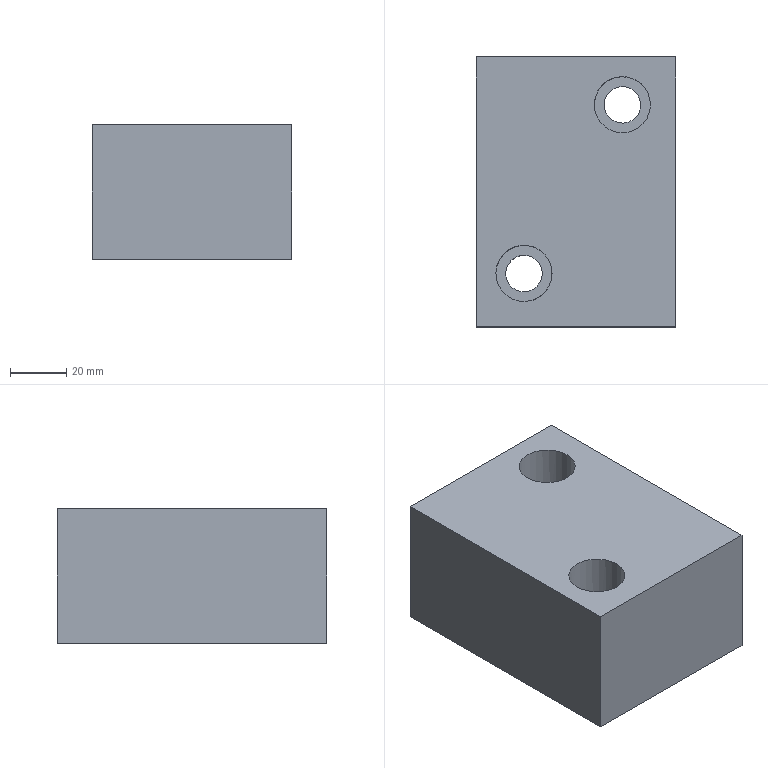Part | STEP file | gslz 2016.10.28-13_id770_x_t | 1 solid | 12 faces | box 71 x 96 x 48 mm | volume 304991 mm3 | plane 8 | cylinder 4 | commonest cylinder face diameters 13 x2 20 x2
STEP:
#1=CARTESIAN_POINT('',(0.,0.,0.));
#2=DIRECTION('',(0.,0.,1.));
#3=DIRECTION('',(1.,0.,0.));
#4=AXIS2_PLACEMENT_3D('',#1,#2,#3);
#5=CARTESIAN_POINT('',(-1464.591,-78.908,-48.));
#6=VERTEX_POINT('',#5);
#7=CARTESIAN_POINT('',(-1463.5,-72.5,-48.));
#8=DIRECTION('',(0.,0.,1.));
#9=DIRECTION('',(-0.1678,-0.9858,0.));
#10=AXIS2_PLACEMENT_3D('',#7,#8,#9);
#11=CIRCLE('',#10,6.5);
#12=CARTESIAN_POINT('',(-1613.5,-26.,-48.));
#13=DIRECTION('',(0.,0.,1.));
#14=DIRECTION('',(0.,1.,0.));
#15=AXIS2_PLACEMENT_3D('',#12,#13,#14);
#16=PLANE('',#15);
#17=CARTESIAN_POINT('',(-46.5,-150.));
#18=DIRECTION('',(-0.9858,0.1678));
#19=AXIS2_PLACEMENT_2D('',#17,#18);
#20=CIRCLE('',#19,6.5);
#21=(GEOMETRIC_REPRESENTATION_CONTEXT(2)PARAMETRIC_REPRESENTATION_CONTEXT()REPRESENTATION_CONTEXT('',''));
#22=DEFINITIONAL_REPRESENTATION('',(#20),#21);
#23=PCURVE('',#16,#22);
#24=CARTESIAN_POINT('',(-1463.5,-72.5,-8.541));
#25=DIRECTION('',(0.,0.,-1.));
#26=DIRECTION('',(-1.,0.,0.));
#27=AXIS2_PLACEMENT_3D('',#24,#25,#26);
#28=CYLINDRICAL_SURFACE('',#27,6.5);
#29=CARTESIAN_POINT('',(11.164,39.459));
#30=DIRECTION('',(-1.,0.));
#31=VECTOR('',#30,1.);
#32=LINE('',#29,#31);
#33=(GEOMETRIC_REPRESENTATION_CONTEXT(2)PARAMETRIC_REPRESENTATION_CONTEXT()REPRESENTATION_CONTEXT('',''));
#34=DEFINITIONAL_REPRESENTATION('',(#32),#33);
#35=PCURVE('',#28,#34);
#36=SURFACE_CURVE('',#11,(#23,#35),.PCURVE_S1.);
#37=EDGE_CURVE('',#6,#6,#36,.T.);
#38=ORIENTED_EDGE('',*,*,#37,.T.);
#39=EDGE_LOOP('',(#38));
#40=FACE_BOUND('',#39,.T.);
#41=CARTESIAN_POINT('',(-1429.591,-18.908,-48.));
#42=VERTEX_POINT('',#41);
#43=CARTESIAN_POINT('',(-1428.5,-12.5,-48.));
#44=DIRECTION('',(0.,0.,1.));
#45=DIRECTION('',(-0.1678,-0.9858,0.));
#46=AXIS2_PLACEMENT_3D('',#43,#44,#45);
#47=CIRCLE('',#46,6.5);
#48=CARTESIAN_POINT('',(13.5,-185.));
#49=DIRECTION('',(-0.9858,0.1678));
#50=AXIS2_PLACEMENT_2D('',#48,#49);
#51=CIRCLE('',#50,6.5);
#52=(GEOMETRIC_REPRESENTATION_CONTEXT(2)PARAMETRIC_REPRESENTATION_CONTEXT()REPRESENTATION_CONTEXT('',''));
#53=DEFINITIONAL_REPRESENTATION('',(#51),#52);
#54=PCURVE('',#16,#53);
#55=CARTESIAN_POINT('',(-1428.5,-12.5,-8.541));
#56=DIRECTION('',(0.,0.,-1.));
#57=DIRECTION('',(-1.,0.,0.));
#58=AXIS2_PLACEMENT_3D('',#55,#56,#57);
#59=CYLINDRICAL_SURFACE('',#58,6.5);
#60=CARTESIAN_POINT('',(11.164,39.459));
#61=DIRECTION('',(-1.,0.));
#62=VECTOR('',#61,1.);
#63=LINE('',#60,#62);
#64=(GEOMETRIC_REPRESENTATION_CONTEXT(2)PARAMETRIC_REPRESENTATION_CONTEXT()REPRESENTATION_CONTEXT('',''));
#65=DEFINITIONAL_REPRESENTATION('',(#63),#64);
#66=PCURVE('',#59,#65);
#67=SURFACE_CURVE('',#47,(#54,#66),.PCURVE_S1.);
#68=EDGE_CURVE('',#42,#42,#67,.T.);
#69=ORIENTED_EDGE('',*,*,#68,.T.);
#70=EDGE_LOOP('',(#69));
#71=FACE_BOUND('',#70,.T.);
#72=CARTESIAN_POINT('',(-1480.5,-91.5,-48.));
#73=VERTEX_POINT('',#72);
#74=CARTESIAN_POINT('',(-1409.5,-91.5,-48.));
#75=VERTEX_POINT('',#74);
#76=CARTESIAN_POINT('',(-1613.5,-91.5,-48.));
#77=DIRECTION('',(1.,0.,0.));
#78=VECTOR('',#77,1.);
#79=LINE('',#76,#78);
#80=CARTESIAN_POINT('',(-65.5,0.));
#81=DIRECTION('',(0.,-1.));
#82=VECTOR('',#81,1.);
#83=LINE('',#80,#82);
#84=(GEOMETRIC_REPRESENTATION_CONTEXT(2)PARAMETRIC_REPRESENTATION_CONTEXT()REPRESENTATION_CONTEXT('',''));
#85=DEFINITIONAL_REPRESENTATION('',(#83),#84);
#86=PCURVE('',#16,#85);
#87=CARTESIAN_POINT('',(-1608.5,-91.5,-43.));
#88=DIRECTION('',(0.,-1.,0.));
#89=DIRECTION('',(0.,0.,1.));
#90=AXIS2_PLACEMENT_3D('',#87,#88,#89);
#91=PLANE('',#90);
#92=CARTESIAN_POINT('',(-5.,5.));
#93=DIRECTION('',(0.,-1.));
#94=VECTOR('',#93,1.);
#95=LINE('',#92,#94);
#96=(GEOMETRIC_REPRESENTATION_CONTEXT(2)PARAMETRIC_REPRESENTATION_CONTEXT()REPRESENTATION_CONTEXT('',''));
#97=DEFINITIONAL_REPRESENTATION('',(#95),#96);
#98=PCURVE('',#91,#97);
#99=SURFACE_CURVE('',#79,(#86,#98),.PCURVE_S1.);
#100=EDGE_CURVE('',#73,#75,#99,.T.);
#101=ORIENTED_EDGE('',*,*,#100,.F.);
#102=CARTESIAN_POINT('',(-1480.5,4.5,-48.));
#103=VERTEX_POINT('',#102);
#104=CARTESIAN_POINT('',(-1480.5,-43.5,-48.));
#105=DIRECTION('',(0.,-1.,0.));
#106=VECTOR('',#105,1.);
#107=LINE('',#104,#106);
#108=CARTESIAN_POINT('',(-17.5,-133.));
#109=DIRECTION('',(-1.,0.));
#110=VECTOR('',#109,1.);
#111=LINE('',#108,#110);
#112=(GEOMETRIC_REPRESENTATION_CONTEXT(2)PARAMETRIC_REPRESENTATION_CONTEXT()REPRESENTATION_CONTEXT('',''));
#113=DEFINITIONAL_REPRESENTATION('',(#111),#112);
#114=PCURVE('',#16,#113);
#115=CARTESIAN_POINT('',(-1480.5,-43.5,-25.5));
#116=DIRECTION('',(1.,0.,0.));
#117=DIRECTION('',(0.,0.,-1.));
#118=AXIS2_PLACEMENT_3D('',#115,#116,#117);
#119=PLANE('',#118);
#120=CARTESIAN_POINT('',(22.5,0.));
#121=DIRECTION('',(0.,-1.));
#122=VECTOR('',#121,1.);
#123=LINE('',#120,#122);
#124=(GEOMETRIC_REPRESENTATION_CONTEXT(2)PARAMETRIC_REPRESENTATION_CONTEXT()REPRESENTATION_CONTEXT('',''));
#125=DEFINITIONAL_REPRESENTATION('',(#123),#124);
#126=PCURVE('',#119,#125);
#127=SURFACE_CURVE('',#107,(#114,#126),.PCURVE_S1.);
#128=EDGE_CURVE('',#103,#73,#127,.T.);
#129=ORIENTED_EDGE('',*,*,#128,.F.);
#130=CARTESIAN_POINT('',(-1409.5,4.5,-48.));
#131=VERTEX_POINT('',#130);
#132=CARTESIAN_POINT('',(-1613.5,4.5,-48.));
#133=DIRECTION('',(-1.,0.,0.));
#134=VECTOR('',#133,1.);
#135=LINE('',#132,#134);
#136=CARTESIAN_POINT('',(30.5,0.));
#137=DIRECTION('',(0.,1.));
#138=VECTOR('',#137,1.);
#139=LINE('',#136,#138);
#140=(GEOMETRIC_REPRESENTATION_CONTEXT(2)PARAMETRIC_REPRESENTATION_CONTEXT()REPRESENTATION_CONTEXT('',''));
#141=DEFINITIONAL_REPRESENTATION('',(#139),#140);
#142=PCURVE('',#16,#141);
#143=CARTESIAN_POINT('',(-1418.5,4.5,-43.));
#144=DIRECTION('',(0.,1.,0.));
#145=DIRECTION('',(-1.,0.,0.));
#146=AXIS2_PLACEMENT_3D('',#143,#144,#145);
#147=PLANE('',#146);
#148=CARTESIAN_POINT('',(195.,-5.));
#149=DIRECTION('',(1.,0.));
#150=VECTOR('',#149,1.);
#151=LINE('',#148,#150);
#152=(GEOMETRIC_REPRESENTATION_CONTEXT(2)PARAMETRIC_REPRESENTATION_CONTEXT()REPRESENTATION_CONTEXT('',''));
#153=DEFINITIONAL_REPRESENTATION('',(#151),#152);
#154=PCURVE('',#147,#153);
#155=SURFACE_CURVE('',#135,(#142,#154),.PCURVE_S1.);
#156=EDGE_CURVE('',#131,#103,#155,.T.);
#157=ORIENTED_EDGE('',*,*,#156,.F.);
#158=CARTESIAN_POINT('',(-1409.5,-26.,-48.));
#159=DIRECTION('',(0.,1.,0.));
#160=VECTOR('',#159,1.);
#161=LINE('',#158,#160);
#162=CARTESIAN_POINT('',(0.,-204.));
#163=DIRECTION('',(1.,0.));
#164=VECTOR('',#163,1.);
#165=LINE('',#162,#164);
#166=(GEOMETRIC_REPRESENTATION_CONTEXT(2)PARAMETRIC_REPRESENTATION_CONTEXT()REPRESENTATION_CONTEXT('',''));
#167=DEFINITIONAL_REPRESENTATION('',(#165),#166);
#168=PCURVE('',#16,#167);
#169=CARTESIAN_POINT('',(-1409.5,-88.5,-43.));
#170=DIRECTION('',(1.,0.,0.));
#171=DIRECTION('',(0.,1.,0.));
#172=AXIS2_PLACEMENT_3D('',#169,#170,#171);
#173=PLANE('',#172);
#174=CARTESIAN_POINT('',(62.5,-5.));
#175=DIRECTION('',(1.,0.));
#176=VECTOR('',#175,1.);
#177=LINE('',#174,#176);
#178=(GEOMETRIC_REPRESENTATION_CONTEXT(2)PARAMETRIC_REPRESENTATION_CONTEXT()REPRESENTATION_CONTEXT('',''));
#179=DEFINITIONAL_REPRESENTATION('',(#177),#178);
#180=PCURVE('',#173,#179);
#181=SURFACE_CURVE('',#161,(#168,#180),.PCURVE_S1.);
#182=EDGE_CURVE('',#75,#131,#181,.T.);
#183=ORIENTED_EDGE('',*,*,#182,.F.);
#184=EDGE_LOOP('',(#101,#129,#157,#183));
#185=FACE_BOUND('',#184,.T.);
#186=ADVANCED_FACE('',(#40,#71,#185),#16,.F.);
#187=CARTESIAN_POINT('',(-1409.5,4.5,0.));
#188=VERTEX_POINT('',#187);
#189=CARTESIAN_POINT('',(-1480.5,4.5,0.));
#190=VERTEX_POINT('',#189);
#191=CARTESIAN_POINT('',(-1418.5,4.5,0.));
#192=DIRECTION('',(-1.,0.,0.));
#193=VECTOR('',#192,1.);
#194=LINE('',#191,#193);
#195=CARTESIAN_POINT('',(0.,43.));
#196=DIRECTION('',(1.,0.));
#197=VECTOR('',#196,1.);
#198=LINE('',#195,#197);
#199=(GEOMETRIC_REPRESENTATION_CONTEXT(2)PARAMETRIC_REPRESENTATION_CONTEXT()REPRESENTATION_CONTEXT('',''));
#200=DEFINITIONAL_REPRESENTATION('',(#198),#199);
#201=PCURVE('',#147,#200);
#202=CARTESIAN_POINT('',(-1517.228,27.5,0.));
#203=DIRECTION('',(0.,0.,1.));
#204=DIRECTION('',(0.,1.,0.));
#205=AXIS2_PLACEMENT_3D('',#202,#203,#204);
#206=PLANE('',#205);
#207=CARTESIAN_POINT('',(-23.,-98.728));
#208=DIRECTION('',(0.,1.));
#209=VECTOR('',#208,1.);
#210=LINE('',#207,#209);
#211=(GEOMETRIC_REPRESENTATION_CONTEXT(2)PARAMETRIC_REPRESENTATION_CONTEXT()REPRESENTATION_CONTEXT('',''));
#212=DEFINITIONAL_REPRESENTATION('',(#210),#211);
#213=PCURVE('',#206,#212);
#214=SURFACE_CURVE('',#194,(#201,#213),.PCURVE_S1.);
#215=EDGE_CURVE('',#188,#190,#214,.T.);
#216=ORIENTED_EDGE('',*,*,#215,.F.);
#217=CARTESIAN_POINT('',(-1409.5,4.5,-43.));
#218=DIRECTION('',(0.,0.,1.));
#219=VECTOR('',#218,1.);
#220=LINE('',#217,#219);
#221=CARTESIAN_POINT('',(-9.,0.));
#222=DIRECTION('',(0.,1.));
#223=VECTOR('',#222,1.);
#224=LINE('',#221,#223);
#225=(GEOMETRIC_REPRESENTATION_CONTEXT(2)PARAMETRIC_REPRESENTATION_CONTEXT()REPRESENTATION_CONTEXT('',''));
#226=DEFINITIONAL_REPRESENTATION('',(#224),#225);
#227=PCURVE('',#147,#226);
#228=CARTESIAN_POINT('',(93.,0.));
#229=DIRECTION('',(0.,1.));
#230=VECTOR('',#229,1.);
#231=LINE('',#228,#230);
#232=(GEOMETRIC_REPRESENTATION_CONTEXT(2)PARAMETRIC_REPRESENTATION_CONTEXT()REPRESENTATION_CONTEXT('',''));
#233=DEFINITIONAL_REPRESENTATION('',(#231),#232);
#234=PCURVE('',#173,#233);
#235=SURFACE_CURVE('',#220,(#227,#234),.PCURVE_S1.);
#236=EDGE_CURVE('',#131,#188,#235,.T.);
#237=ORIENTED_EDGE('',*,*,#236,.F.);
#238=ORIENTED_EDGE('',*,*,#156,.T.);
#239=CARTESIAN_POINT('',(-1480.5,4.5,-43.));
#240=DIRECTION('',(0.,0.,-1.));
#241=VECTOR('',#240,1.);
#242=LINE('',#239,#241);
#243=CARTESIAN_POINT('',(62.,0.));
#244=DIRECTION('',(0.,-1.));
#245=VECTOR('',#244,1.);
#246=LINE('',#243,#245);
#247=(GEOMETRIC_REPRESENTATION_CONTEXT(2)PARAMETRIC_REPRESENTATION_CONTEXT()REPRESENTATION_CONTEXT('',''));
#248=DEFINITIONAL_REPRESENTATION('',(#246),#247);
#249=PCURVE('',#147,#248);
#250=CARTESIAN_POINT('',(17.5,48.));
#251=DIRECTION('',(1.,0.));
#252=VECTOR('',#251,1.);
#253=LINE('',#250,#252);
#254=(GEOMETRIC_REPRESENTATION_CONTEXT(2)PARAMETRIC_REPRESENTATION_CONTEXT()REPRESENTATION_CONTEXT('',''));
#255=DEFINITIONAL_REPRESENTATION('',(#253),#254);
#256=PCURVE('',#119,#255);
#257=SURFACE_CURVE('',#242,(#249,#256),.PCURVE_S1.);
#258=EDGE_CURVE('',#190,#103,#257,.T.);
#259=ORIENTED_EDGE('',*,*,#258,.F.);
#260=EDGE_LOOP('',(#216,#237,#238,#259));
#261=FACE_BOUND('',#260,.T.);
#262=ADVANCED_FACE('',(#261),#147,.T.);
#263=CARTESIAN_POINT('',(-1409.5,-91.5,0.));
#264=VERTEX_POINT('',#263);
#265=CARTESIAN_POINT('',(-1409.5,-88.5,0.));
#266=DIRECTION('',(0.,1.,0.));
#267=VECTOR('',#266,1.);
#268=LINE('',#265,#267);
#269=CARTESIAN_POINT('',(0.,43.));
#270=DIRECTION('',(1.,0.));
#271=VECTOR('',#270,1.);
#272=LINE('',#269,#271);
#273=(GEOMETRIC_REPRESENTATION_CONTEXT(2)PARAMETRIC_REPRESENTATION_CONTEXT()REPRESENTATION_CONTEXT('',''));
#274=DEFINITIONAL_REPRESENTATION('',(#272),#273);
#275=PCURVE('',#173,#274);
#276=CARTESIAN_POINT('',(-116.,-107.728));
#277=DIRECTION('',(1.,0.));
#278=VECTOR('',#277,1.);
#279=LINE('',#276,#278);
#280=(GEOMETRIC_REPRESENTATION_CONTEXT(2)PARAMETRIC_REPRESENTATION_CONTEXT()REPRESENTATION_CONTEXT('',''));
#281=DEFINITIONAL_REPRESENTATION('',(#279),#280);
#282=PCURVE('',#206,#281);
#283=SURFACE_CURVE('',#268,(#275,#282),.PCURVE_S1.);
#284=EDGE_CURVE('',#264,#188,#283,.T.);
#285=ORIENTED_EDGE('',*,*,#284,.F.);
#286=CARTESIAN_POINT('',(-1409.5,-91.5,-43.));
#287=DIRECTION('',(0.,0.,1.));
#288=VECTOR('',#287,1.);
#289=LINE('',#286,#288);
#290=CARTESIAN_POINT('',(-3.,0.));
#291=DIRECTION('',(0.,1.));
#292=VECTOR('',#291,1.);
#293=LINE('',#290,#292);
#294=(GEOMETRIC_REPRESENTATION_CONTEXT(2)PARAMETRIC_REPRESENTATION_CONTEXT()REPRESENTATION_CONTEXT('',''));
#295=DEFINITIONAL_REPRESENTATION('',(#293),#294);
#296=PCURVE('',#173,#295);
#297=CARTESIAN_POINT('',(0.,-199.));
#298=DIRECTION('',(1.,0.));
#299=VECTOR('',#298,1.);
#300=LINE('',#297,#299);
#301=(GEOMETRIC_REPRESENTATION_CONTEXT(2)PARAMETRIC_REPRESENTATION_CONTEXT()REPRESENTATION_CONTEXT('',''));
#302=DEFINITIONAL_REPRESENTATION('',(#300),#301);
#303=PCURVE('',#91,#302);
#304=SURFACE_CURVE('',#289,(#296,#303),.PCURVE_S1.);
#305=EDGE_CURVE('',#75,#264,#304,.T.);
#306=ORIENTED_EDGE('',*,*,#305,.F.);
#307=ORIENTED_EDGE('',*,*,#182,.T.);
#308=ORIENTED_EDGE('',*,*,#236,.T.);
#309=EDGE_LOOP('',(#285,#306,#307,#308));
#310=FACE_BOUND('',#309,.T.);
#311=ADVANCED_FACE('',(#310),#173,.T.);
#312=CARTESIAN_POINT('',(-1480.5,-91.5,0.));
#313=VERTEX_POINT('',#312);
#314=CARTESIAN_POINT('',(-1480.5,-91.5,-43.));
#315=DIRECTION('',(0.,0.,-1.));
#316=VECTOR('',#315,1.);
#317=LINE('',#314,#316);
#318=CARTESIAN_POINT('',(0.,-128.));
#319=DIRECTION('',(-1.,0.));
#320=VECTOR('',#319,1.);
#321=LINE('',#318,#320);
#322=(GEOMETRIC_REPRESENTATION_CONTEXT(2)PARAMETRIC_REPRESENTATION_CONTEXT()REPRESENTATION_CONTEXT('',''));
#323=DEFINITIONAL_REPRESENTATION('',(#321),#322);
#324=PCURVE('',#91,#323);
#325=CARTESIAN_POINT('',(17.5,-48.));
#326=DIRECTION('',(1.,0.));
#327=VECTOR('',#326,1.);
#328=LINE('',#325,#327);
#329=(GEOMETRIC_REPRESENTATION_CONTEXT(2)PARAMETRIC_REPRESENTATION_CONTEXT()REPRESENTATION_CONTEXT('',''));
#330=DEFINITIONAL_REPRESENTATION('',(#328),#329);
#331=PCURVE('',#119,#330);
#332=SURFACE_CURVE('',#317,(#324,#331),.PCURVE_S1.);
#333=EDGE_CURVE('',#313,#73,#332,.T.);
#334=ORIENTED_EDGE('',*,*,#333,.T.);
#335=ORIENTED_EDGE('',*,*,#100,.T.);
#336=ORIENTED_EDGE('',*,*,#305,.T.);
#337=CARTESIAN_POINT('',(-1608.5,-91.5,0.));
#338=DIRECTION('',(1.,0.,0.));
#339=VECTOR('',#338,1.);
#340=LINE('',#337,#339);
#341=CARTESIAN_POINT('',(43.,0.));
#342=DIRECTION('',(0.,-1.));
#343=VECTOR('',#342,1.);
#344=LINE('',#341,#343);
#345=(GEOMETRIC_REPRESENTATION_CONTEXT(2)PARAMETRIC_REPRESENTATION_CONTEXT()REPRESENTATION_CONTEXT('',''));
#346=DEFINITIONAL_REPRESENTATION('',(#344),#345);
#347=PCURVE('',#91,#346);
#348=CARTESIAN_POINT('',(-119.,91.272));
#349=DIRECTION('',(0.,-1.));
#350=VECTOR('',#349,1.);
#351=LINE('',#348,#350);
#352=(GEOMETRIC_REPRESENTATION_CONTEXT(2)PARAMETRIC_REPRESENTATION_CONTEXT()REPRESENTATION_CONTEXT('',''));
#353=DEFINITIONAL_REPRESENTATION('',(#351),#352);
#354=PCURVE('',#206,#353);
#355=SURFACE_CURVE('',#340,(#347,#354),.PCURVE_S1.);
#356=EDGE_CURVE('',#313,#264,#355,.T.);
#357=ORIENTED_EDGE('',*,*,#356,.F.);
#358=EDGE_LOOP('',(#334,#335,#336,#357));
#359=FACE_BOUND('',#358,.T.);
#360=ADVANCED_FACE('',(#359),#91,.T.);
#361=ORIENTED_EDGE('',*,*,#333,.F.);
#362=CARTESIAN_POINT('',(-1480.5,27.5,0.));
#363=DIRECTION('',(0.,1.,0.));
#364=VECTOR('',#363,1.);
#365=LINE('',#362,#364);
#366=CARTESIAN_POINT('',(-25.5,71.));
#367=DIRECTION('',(0.,1.));
#368=VECTOR('',#367,1.);
#369=LINE('',#366,#368);
#370=(GEOMETRIC_REPRESENTATION_CONTEXT(2)PARAMETRIC_REPRESENTATION_CONTEXT()REPRESENTATION_CONTEXT('',''));
#371=DEFINITIONAL_REPRESENTATION('',(#369),#370);
#372=PCURVE('',#119,#371);
#373=CARTESIAN_POINT('',(0.,-36.728));
#374=DIRECTION('',(1.,0.));
#375=VECTOR('',#374,1.);
#376=LINE('',#373,#375);
#377=(GEOMETRIC_REPRESENTATION_CONTEXT(2)PARAMETRIC_REPRESENTATION_CONTEXT()REPRESENTATION_CONTEXT('',''));
#378=DEFINITIONAL_REPRESENTATION('',(#376),#377);
#379=PCURVE('',#206,#378);
#380=SURFACE_CURVE('',#365,(#372,#379),.PCURVE_S1.);
#381=EDGE_CURVE('',#313,#190,#380,.T.);
#382=ORIENTED_EDGE('',*,*,#381,.T.);
#383=ORIENTED_EDGE('',*,*,#258,.T.);
#384=ORIENTED_EDGE('',*,*,#128,.T.);
#385=EDGE_LOOP('',(#361,#382,#383,#384));
#386=FACE_BOUND('',#385,.T.);
#387=ADVANCED_FACE('',(#386),#119,.F.);
#388=CARTESIAN_POINT('',(-1453.5,-72.5,0.));
#389=VERTEX_POINT('',#388);
#390=CARTESIAN_POINT('',(-1465.178,-82.358,0.));
#391=VERTEX_POINT('',#390);
#392=CARTESIAN_POINT('',(-1463.5,-72.5,0.));
#393=DIRECTION('',(0.,0.,1.));
#394=DIRECTION('',(1.,0.,0.));
#395=AXIS2_PLACEMENT_3D('',#392,#393,#394);
#396=CIRCLE('',#395,10.);
#397=CARTESIAN_POINT('',(-100.,-53.728));
#398=DIRECTION('',(0.,-1.));
#399=AXIS2_PLACEMENT_2D('',#397,#398);
#400=CIRCLE('',#399,10.);
#401=(GEOMETRIC_REPRESENTATION_CONTEXT(2)PARAMETRIC_REPRESENTATION_CONTEXT()REPRESENTATION_CONTEXT('',''));
#402=DEFINITIONAL_REPRESENTATION('',(#400),#401);
#403=PCURVE('',#206,#402);
#404=CARTESIAN_POINT('',(-1463.5,-72.5,-8.541));
#405=DIRECTION('',(0.,0.,-1.));
#406=DIRECTION('',(-1.,0.,0.));
#407=AXIS2_PLACEMENT_3D('',#404,#405,#406);
#408=CYLINDRICAL_SURFACE('',#407,10.);
#409=CARTESIAN_POINT('',(9.425,-8.541));
#410=DIRECTION('',(-1.,0.));
#411=VECTOR('',#410,1.);
#412=LINE('',#409,#411);
#413=(GEOMETRIC_REPRESENTATION_CONTEXT(2)PARAMETRIC_REPRESENTATION_CONTEXT()REPRESENTATION_CONTEXT('',''));
#414=DEFINITIONAL_REPRESENTATION('',(#412),#413);
#415=PCURVE('',#408,#414);
#416=SURFACE_CURVE('',#396,(#403,#415),.PCURVE_S1.);
#417=EDGE_CURVE('',#389,#391,#416,.T.);
#418=ORIENTED_EDGE('',*,*,#417,.F.);
#419=CARTESIAN_POINT('',(-1463.5,-72.5,0.));
#420=DIRECTION('',(0.,0.,1.));
#421=DIRECTION('',(1.,0.,0.));
#422=AXIS2_PLACEMENT_3D('',#419,#420,#421);
#423=CIRCLE('',#422,10.);
#424=CARTESIAN_POINT('',(-100.,-53.728));
#425=DIRECTION('',(0.,-1.));
#426=AXIS2_PLACEMENT_2D('',#424,#425);
#427=CIRCLE('',#426,10.);
#428=(GEOMETRIC_REPRESENTATION_CONTEXT(2)PARAMETRIC_REPRESENTATION_CONTEXT()REPRESENTATION_CONTEXT('',''));
#429=DEFINITIONAL_REPRESENTATION('',(#427),#428);
#430=PCURVE('',#206,#429);
#431=CARTESIAN_POINT('',(15.708,-8.541));
#432=DIRECTION('',(-1.,0.));
#433=VECTOR('',#432,1.);
#434=LINE('',#431,#433);
#435=(GEOMETRIC_REPRESENTATION_CONTEXT(2)PARAMETRIC_REPRESENTATION_CONTEXT()REPRESENTATION_CONTEXT('',''));
#436=DEFINITIONAL_REPRESENTATION('',(#434),#435);
#437=PCURVE('',#408,#436);
#438=SURFACE_CURVE('',#423,(#430,#437),.PCURVE_S1.);
#439=EDGE_CURVE('',#391,#389,#438,.T.);
#440=ORIENTED_EDGE('',*,*,#439,.F.);
#441=EDGE_LOOP('',(#418,#440));
#442=FACE_BOUND('',#441,.T.);
#443=CARTESIAN_POINT('',(-1418.5,-12.5,0.));
#444=VERTEX_POINT('',#443);
#445=CARTESIAN_POINT('',(-1430.178,-22.358,0.));
#446=VERTEX_POINT('',#445);
#447=CARTESIAN_POINT('',(-1428.5,-12.5,0.));
#448=DIRECTION('',(0.,0.,1.));
#449=DIRECTION('',(1.,0.,0.));
#450=AXIS2_PLACEMENT_3D('',#447,#448,#449);
#451=CIRCLE('',#450,10.);
#452=CARTESIAN_POINT('',(-40.,-88.728));
#453=DIRECTION('',(0.,-1.));
#454=AXIS2_PLACEMENT_2D('',#452,#453);
#455=CIRCLE('',#454,10.);
#456=(GEOMETRIC_REPRESENTATION_CONTEXT(2)PARAMETRIC_REPRESENTATION_CONTEXT()REPRESENTATION_CONTEXT('',''));
#457=DEFINITIONAL_REPRESENTATION('',(#455),#456);
#458=PCURVE('',#206,#457);
#459=CARTESIAN_POINT('',(-1428.5,-12.5,-8.541));
#460=DIRECTION('',(0.,0.,-1.));
#461=DIRECTION('',(-1.,0.,0.));
#462=AXIS2_PLACEMENT_3D('',#459,#460,#461);
#463=CYLINDRICAL_SURFACE('',#462,10.);
#464=CARTESIAN_POINT('',(9.425,-8.541));
#465=DIRECTION('',(-1.,0.));
#466=VECTOR('',#465,1.);
#467=LINE('',#464,#466);
#468=(GEOMETRIC_REPRESENTATION_CONTEXT(2)PARAMETRIC_REPRESENTATION_CONTEXT()REPRESENTATION_CONTEXT('',''));
#469=DEFINITIONAL_REPRESENTATION('',(#467),#468);
#470=PCURVE('',#463,#469);
#471=SURFACE_CURVE('',#451,(#458,#470),.PCURVE_S1.);
#472=EDGE_CURVE('',#444,#446,#471,.T.);
#473=ORIENTED_EDGE('',*,*,#472,.F.);
#474=CARTESIAN_POINT('',(-1428.5,-12.5,0.));
#475=DIRECTION('',(0.,0.,1.));
#476=DIRECTION('',(1.,0.,0.));
#477=AXIS2_PLACEMENT_3D('',#474,#475,#476);
#478=CIRCLE('',#477,10.);
#479=CARTESIAN_POINT('',(-40.,-88.728));
#480=DIRECTION('',(0.,-1.));
#481=AXIS2_PLACEMENT_2D('',#479,#480);
#482=CIRCLE('',#481,10.);
#483=(GEOMETRIC_REPRESENTATION_CONTEXT(2)PARAMETRIC_REPRESENTATION_CONTEXT()REPRESENTATION_CONTEXT('',''));
#484=DEFINITIONAL_REPRESENTATION('',(#482),#483);
#485=PCURVE('',#206,#484);
#486=CARTESIAN_POINT('',(15.708,-8.541));
#487=DIRECTION('',(-1.,0.));
#488=VECTOR('',#487,1.);
#489=LINE('',#486,#488);
#490=(GEOMETRIC_REPRESENTATION_CONTEXT(2)PARAMETRIC_REPRESENTATION_CONTEXT()REPRESENTATION_CONTEXT('',''));
#491=DEFINITIONAL_REPRESENTATION('',(#489),#490);
#492=PCURVE('',#463,#491);
#493=SURFACE_CURVE('',#478,(#485,#492),.PCURVE_S1.);
#494=EDGE_CURVE('',#446,#444,#493,.T.);
#495=ORIENTED_EDGE('',*,*,#494,.F.);
#496=EDGE_LOOP('',(#473,#495));
#497=FACE_BOUND('',#496,.T.);
#498=ORIENTED_EDGE('',*,*,#381,.F.);
#499=ORIENTED_EDGE('',*,*,#356,.T.);
#500=ORIENTED_EDGE('',*,*,#284,.T.);
#501=ORIENTED_EDGE('',*,*,#215,.T.);
#502=EDGE_LOOP('',(#498,#499,#500,#501));
#503=FACE_BOUND('',#502,.T.);
#504=ADVANCED_FACE('',(#442,#497,#503),#206,.T.);
#505=CARTESIAN_POINT('',(-1429.591,-18.908,-26.));
#506=VERTEX_POINT('',#505);
#507=CARTESIAN_POINT('',(-1428.5,-12.5,-26.));
#508=DIRECTION('',(0.,0.,1.));
#509=DIRECTION('',(-0.1678,-0.9858,0.));
#510=AXIS2_PLACEMENT_3D('',#507,#508,#509);
#511=CIRCLE('',#510,6.5);
#512=CARTESIAN_POINT('',(-1428.5,-12.5,-26.));
#513=DIRECTION('',(0.,0.,1.));
#514=DIRECTION('',(-0.1678,-0.9858,0.));
#515=AXIS2_PLACEMENT_3D('',#512,#513,#514);
#516=PLANE('',#515);
#517=CARTESIAN_POINT('',(0.,0.));
#518=DIRECTION('',(1.,0.));
#519=AXIS2_PLACEMENT_2D('',#517,#518);
#520=CIRCLE('',#519,6.5);
#521=(GEOMETRIC_REPRESENTATION_CONTEXT(2)PARAMETRIC_REPRESENTATION_CONTEXT()REPRESENTATION_CONTEXT('',''));
#522=DEFINITIONAL_REPRESENTATION('',(#520),#521);
#523=PCURVE('',#516,#522);
#524=CARTESIAN_POINT('',(11.164,17.459));
#525=DIRECTION('',(-1.,0.));
#526=VECTOR('',#525,1.);
#527=LINE('',#524,#526);
#528=(GEOMETRIC_REPRESENTATION_CONTEXT(2)PARAMETRIC_REPRESENTATION_CONTEXT()REPRESENTATION_CONTEXT('',''));
#529=DEFINITIONAL_REPRESENTATION('',(#527),#528);
#530=PCURVE('',#59,#529);
#531=SURFACE_CURVE('',#511,(#523,#530),.PCURVE_S1.);
#532=EDGE_CURVE('',#506,#506,#531,.T.);
#533=ORIENTED_EDGE('',*,*,#532,.F.);
#534=EDGE_LOOP('',(#533));
#535=FACE_BOUND('',#534,.T.);
#536=CARTESIAN_POINT('',(-1430.178,-22.358,-26.));
#537=VERTEX_POINT('',#536);
#538=CARTESIAN_POINT('',(-1428.5,-12.5,-26.));
#539=DIRECTION('',(0.,0.,-1.));
#540=DIRECTION('',(-0.1678,-0.9858,0.));
#541=AXIS2_PLACEMENT_3D('',#538,#539,#540);
#542=CIRCLE('',#541,10.);
#543=CARTESIAN_POINT('',(10.,0.));
#544=CARTESIAN_POINT('',(10.,-17.321));
#545=CARTESIAN_POINT('',(-5.,-8.66));
#546=CARTESIAN_POINT('',(-20.,0.));
#547=CARTESIAN_POINT('',(-5.,8.66));
#548=CARTESIAN_POINT('',(10.,17.321));
#549=CARTESIAN_POINT('',(10.,0.));
#550=(BOUNDED_CURVE()B_SPLINE_CURVE(2,(#543,#544,#545,#546,#547,#548,#549),.UNSPECIFIED.,.T.,.F.)B_SPLINE_CURVE_WITH_KNOTS((1,2,2,2,2,1),(-2.094,0.,2.094,4.189,6.283,8.378),.UNSPECIFIED.)CURVE()GEOMETRIC_REPRESENTATION_ITEM()RATIONAL_B_SPLINE_CURVE((1.,0.5,1.,0.5,1.,0.5,1.))REPRESENTATION_ITEM(''));
#551=(GEOMETRIC_REPRESENTATION_CONTEXT(2)PARAMETRIC_REPRESENTATION_CONTEXT()REPRESENTATION_CONTEXT('',''));
#552=DEFINITIONAL_REPRESENTATION('',(#550),#551);
#553=PCURVE('',#516,#552);
#554=CARTESIAN_POINT('',(4.881,17.459));
#555=DIRECTION('',(1.,0.));
#556=VECTOR('',#555,1.);
#557=LINE('',#554,#556);
#558=(GEOMETRIC_REPRESENTATION_CONTEXT(2)PARAMETRIC_REPRESENTATION_CONTEXT()REPRESENTATION_CONTEXT('',''));
#559=DEFINITIONAL_REPRESENTATION('',(#557),#558);
#560=PCURVE('',#463,#559);
#561=SURFACE_CURVE('',#542,(#553,#560),.PCURVE_S1.);
#562=EDGE_CURVE('',#537,#537,#561,.T.);
#563=ORIENTED_EDGE('',*,*,#562,.F.);
#564=EDGE_LOOP('',(#563));
#565=FACE_BOUND('',#564,.T.);
#566=ADVANCED_FACE('',(#535,#565),#516,.T.);
#567=ORIENTED_EDGE('',*,*,#494,.F.);
#568=CARTESIAN_POINT('',(-1430.178,-22.358,0.));
#569=CARTESIAN_POINT('',(-1430.178,-22.358,-26.));
#570=B_SPLINE_CURVE_WITH_KNOTS('',1,(#568,#569),.UNSPECIFIED.,.F.,.F.,(2,2),(-8.541,17.459),.PIECEWISE_BEZIER_KNOTS.);
#571=CARTESIAN_POINT('',(11.164,0.));
#572=DIRECTION('',(0.,1.));
#573=VECTOR('',#572,1.);
#574=LINE('',#571,#573);
#575=(GEOMETRIC_REPRESENTATION_CONTEXT(2)PARAMETRIC_REPRESENTATION_CONTEXT()REPRESENTATION_CONTEXT('',''));
#576=DEFINITIONAL_REPRESENTATION('',(#574),#575);
#577=PCURVE('',#463,#576);
#578=CARTESIAN_POINT('',(4.881,0.));
#579=DIRECTION('',(0.,1.));
#580=VECTOR('',#579,1.);
#581=LINE('',#578,#580);
#582=(GEOMETRIC_REPRESENTATION_CONTEXT(2)PARAMETRIC_REPRESENTATION_CONTEXT()REPRESENTATION_CONTEXT('',''));
#583=DEFINITIONAL_REPRESENTATION('',(#581),#582);
#584=PCURVE('',#463,#583);
#585=SEAM_CURVE('',#570,(#577,#584),.PCURVE_S1.);
#586=EDGE_CURVE('',#446,#537,#585,.T.);
#587=ORIENTED_EDGE('',*,*,#586,.T.);
#588=ORIENTED_EDGE('',*,*,#562,.F.);
#589=ORIENTED_EDGE('',*,*,#586,.F.);
#590=ORIENTED_EDGE('',*,*,#472,.F.);
#591=EDGE_LOOP('',(#567,#587,#588,#589,#590));
#592=FACE_BOUND('',#591,.F.);
#593=ADVANCED_FACE('',(#592),#463,.F.);
#594=ORIENTED_EDGE('',*,*,#532,.F.);
#595=CARTESIAN_POINT('',(-1429.591,-18.908,-26.));
#596=CARTESIAN_POINT('',(-1429.591,-18.908,-48.));
#597=B_SPLINE_CURVE_WITH_KNOTS('',1,(#595,#596),.UNSPECIFIED.,.F.,.F.,(2,2),(17.459,39.459),.PIECEWISE_BEZIER_KNOTS.);
#598=CARTESIAN_POINT('',(11.164,0.));
#599=DIRECTION('',(0.,1.));
#600=VECTOR('',#599,1.);
#601=LINE('',#598,#600);
#602=(GEOMETRIC_REPRESENTATION_CONTEXT(2)PARAMETRIC_REPRESENTATION_CONTEXT()REPRESENTATION_CONTEXT('',''));
#603=DEFINITIONAL_REPRESENTATION('',(#601),#602);
#604=PCURVE('',#59,#603);
#605=CARTESIAN_POINT('',(4.881,0.));
#606=DIRECTION('',(0.,1.));
#607=VECTOR('',#606,1.);
#608=LINE('',#605,#607);
#609=(GEOMETRIC_REPRESENTATION_CONTEXT(2)PARAMETRIC_REPRESENTATION_CONTEXT()REPRESENTATION_CONTEXT('',''));
#610=DEFINITIONAL_REPRESENTATION('',(#608),#609);
#611=PCURVE('',#59,#610);
#612=SEAM_CURVE('',#597,(#604,#611),.PCURVE_S1.);
#613=EDGE_CURVE('',#506,#42,#612,.T.);
#614=ORIENTED_EDGE('',*,*,#613,.T.);
#615=ORIENTED_EDGE('',*,*,#68,.T.);
#616=ORIENTED_EDGE('',*,*,#613,.F.);
#617=EDGE_LOOP('',(#594,#614,#615,#616));
#618=FACE_BOUND('',#617,.F.);
#619=ADVANCED_FACE('',(#618),#59,.F.);
#620=CARTESIAN_POINT('',(-1464.591,-78.908,-26.));
#621=VERTEX_POINT('',#620);
#622=CARTESIAN_POINT('',(-1463.5,-72.5,-26.));
#623=DIRECTION('',(0.,0.,1.));
#624=DIRECTION('',(-0.1678,-0.9858,0.));
#625=AXIS2_PLACEMENT_3D('',#622,#623,#624);
#626=CIRCLE('',#625,6.5);
#627=CARTESIAN_POINT('',(-1463.5,-72.5,-26.));
#628=DIRECTION('',(0.,0.,1.));
#629=DIRECTION('',(-0.1678,-0.9858,0.));
#630=AXIS2_PLACEMENT_3D('',#627,#628,#629);
#631=PLANE('',#630);
#632=CARTESIAN_POINT('',(0.,0.));
#633=DIRECTION('',(1.,0.));
#634=AXIS2_PLACEMENT_2D('',#632,#633);
#635=CIRCLE('',#634,6.5);
#636=(GEOMETRIC_REPRESENTATION_CONTEXT(2)PARAMETRIC_REPRESENTATION_CONTEXT()REPRESENTATION_CONTEXT('',''));
#637=DEFINITIONAL_REPRESENTATION('',(#635),#636);
#638=PCURVE('',#631,#637);
#639=CARTESIAN_POINT('',(11.164,17.459));
#640=DIRECTION('',(-1.,0.));
#641=VECTOR('',#640,1.);
#642=LINE('',#639,#641);
#643=(GEOMETRIC_REPRESENTATION_CONTEXT(2)PARAMETRIC_REPRESENTATION_CONTEXT()REPRESENTATION_CONTEXT('',''));
#644=DEFINITIONAL_REPRESENTATION('',(#642),#643);
#645=PCURVE('',#28,#644);
#646=SURFACE_CURVE('',#626,(#638,#645),.PCURVE_S1.);
#647=EDGE_CURVE('',#621,#621,#646,.T.);
#648=ORIENTED_EDGE('',*,*,#647,.F.);
#649=EDGE_LOOP('',(#648));
#650=FACE_BOUND('',#649,.T.);
#651=CARTESIAN_POINT('',(-1465.178,-82.358,-26.));
#652=VERTEX_POINT('',#651);
#653=CARTESIAN_POINT('',(-1463.5,-72.5,-26.));
#654=DIRECTION('',(0.,0.,-1.));
#655=DIRECTION('',(-0.1678,-0.9858,0.));
#656=AXIS2_PLACEMENT_3D('',#653,#654,#655);
#657=CIRCLE('',#656,10.);
#658=CARTESIAN_POINT('',(10.,0.));
#659=CARTESIAN_POINT('',(10.,-17.321));
#660=CARTESIAN_POINT('',(-5.,-8.66));
#661=CARTESIAN_POINT('',(-20.,0.));
#662=CARTESIAN_POINT('',(-5.,8.66));
#663=CARTESIAN_POINT('',(10.,17.321));
#664=CARTESIAN_POINT('',(10.,0.));
#665=(BOUNDED_CURVE()B_SPLINE_CURVE(2,(#658,#659,#660,#661,#662,#663,#664),.UNSPECIFIED.,.T.,.F.)B_SPLINE_CURVE_WITH_KNOTS((1,2,2,2,2,1),(-2.094,0.,2.094,4.189,6.283,8.378),.UNSPECIFIED.)CURVE()GEOMETRIC_REPRESENTATION_ITEM()RATIONAL_B_SPLINE_CURVE((1.,0.5,1.,0.5,1.,0.5,1.))REPRESENTATION_ITEM(''));
#666=(GEOMETRIC_REPRESENTATION_CONTEXT(2)PARAMETRIC_REPRESENTATION_CONTEXT()REPRESENTATION_CONTEXT('',''));
#667=DEFINITIONAL_REPRESENTATION('',(#665),#666);
#668=PCURVE('',#631,#667);
#669=CARTESIAN_POINT('',(4.881,17.459));
#670=DIRECTION('',(1.,0.));
#671=VECTOR('',#670,1.);
#672=LINE('',#669,#671);
#673=(GEOMETRIC_REPRESENTATION_CONTEXT(2)PARAMETRIC_REPRESENTATION_CONTEXT()REPRESENTATION_CONTEXT('',''));
#674=DEFINITIONAL_REPRESENTATION('',(#672),#673);
#675=PCURVE('',#408,#674);
#676=SURFACE_CURVE('',#657,(#668,#675),.PCURVE_S1.);
#677=EDGE_CURVE('',#652,#652,#676,.T.);
#678=ORIENTED_EDGE('',*,*,#677,.F.);
#679=EDGE_LOOP('',(#678));
#680=FACE_BOUND('',#679,.T.);
#681=ADVANCED_FACE('',(#650,#680),#631,.T.);
#682=ORIENTED_EDGE('',*,*,#439,.F.);
#683=CARTESIAN_POINT('',(-1465.178,-82.358,0.));
#684=CARTESIAN_POINT('',(-1465.178,-82.358,-26.));
#685=B_SPLINE_CURVE_WITH_KNOTS('',1,(#683,#684),.UNSPECIFIED.,.F.,.F.,(2,2),(-8.541,17.459),.PIECEWISE_BEZIER_KNOTS.);
#686=CARTESIAN_POINT('',(11.164,0.));
#687=DIRECTION('',(0.,1.));
#688=VECTOR('',#687,1.);
#689=LINE('',#686,#688);
#690=(GEOMETRIC_REPRESENTATION_CONTEXT(2)PARAMETRIC_REPRESENTATION_CONTEXT()REPRESENTATION_CONTEXT('',''));
#691=DEFINITIONAL_REPRESENTATION('',(#689),#690);
#692=PCURVE('',#408,#691);
#693=CARTESIAN_POINT('',(4.881,0.));
#694=DIRECTION('',(0.,1.));
#695=VECTOR('',#694,1.);
#696=LINE('',#693,#695);
#697=(GEOMETRIC_REPRESENTATION_CONTEXT(2)PARAMETRIC_REPRESENTATION_CONTEXT()REPRESENTATION_CONTEXT('',''));
#698=DEFINITIONAL_REPRESENTATION('',(#696),#697);
#699=PCURVE('',#408,#698);
#700=SEAM_CURVE('',#685,(#692,#699),.PCURVE_S1.);
#701=EDGE_CURVE('',#391,#652,#700,.T.);
#702=ORIENTED_EDGE('',*,*,#701,.T.);
#703=ORIENTED_EDGE('',*,*,#677,.F.);
#704=ORIENTED_EDGE('',*,*,#701,.F.);
#705=ORIENTED_EDGE('',*,*,#417,.F.);
#706=EDGE_LOOP('',(#682,#702,#703,#704,#705));
#707=FACE_BOUND('',#706,.F.);
#708=ADVANCED_FACE('',(#707),#408,.F.);
#709=ORIENTED_EDGE('',*,*,#647,.F.);
#710=CARTESIAN_POINT('',(-1464.591,-78.908,-26.));
#711=CARTESIAN_POINT('',(-1464.591,-78.908,-48.));
#712=B_SPLINE_CURVE_WITH_KNOTS('',1,(#710,#711),.UNSPECIFIED.,.F.,.F.,(2,2),(17.459,39.459),.PIECEWISE_BEZIER_KNOTS.);
#713=CARTESIAN_POINT('',(11.164,0.));
#714=DIRECTION('',(0.,1.));
#715=VECTOR('',#714,1.);
#716=LINE('',#713,#715);
#717=(GEOMETRIC_REPRESENTATION_CONTEXT(2)PARAMETRIC_REPRESENTATION_CONTEXT()REPRESENTATION_CONTEXT('',''));
#718=DEFINITIONAL_REPRESENTATION('',(#716),#717);
#719=PCURVE('',#28,#718);
#720=CARTESIAN_POINT('',(4.881,0.));
#721=DIRECTION('',(0.,1.));
#722=VECTOR('',#721,1.);
#723=LINE('',#720,#722);
#724=(GEOMETRIC_REPRESENTATION_CONTEXT(2)PARAMETRIC_REPRESENTATION_CONTEXT()REPRESENTATION_CONTEXT('',''));
#725=DEFINITIONAL_REPRESENTATION('',(#723),#724);
#726=PCURVE('',#28,#725);
#727=SEAM_CURVE('',#712,(#719,#726),.PCURVE_S1.);
#728=EDGE_CURVE('',#621,#6,#727,.T.);
#729=ORIENTED_EDGE('',*,*,#728,.T.);
#730=ORIENTED_EDGE('',*,*,#37,.T.);
#731=ORIENTED_EDGE('',*,*,#728,.F.);
#732=EDGE_LOOP('',(#709,#729,#730,#731));
#733=FACE_BOUND('',#732,.F.);
#734=ADVANCED_FACE('',(#733),#28,.F.);
#735=CLOSED_SHELL('',(#186,#262,#311,#360,#387,#504,#566,#593,#619,#681,#708,#734));
#736=MANIFOLD_SOLID_BREP('',#735);
#737=(LENGTH_UNIT()NAMED_UNIT(*)SI_UNIT(.MILLI.,.METRE.));
#738=UNCERTAINTY_MEASURE_WITH_UNIT(LENGTH_MEASURE(0.000005),#737,'','');
#739=(NAMED_UNIT(*)PLANE_ANGLE_UNIT()SI_UNIT($,.RADIAN.));
#740=(NAMED_UNIT(*)SI_UNIT($,.STERADIAN.)SOLID_ANGLE_UNIT());
#741=(GEOMETRIC_REPRESENTATION_CONTEXT(3)GLOBAL_UNCERTAINTY_ASSIGNED_CONTEXT((#738))GLOBAL_UNIT_ASSIGNED_CONTEXT((#737,#739,#740))REPRESENTATION_CONTEXT('',''));
#742=ADVANCED_BREP_SHAPE_REPRESENTATION('',(#4,#736),#741);